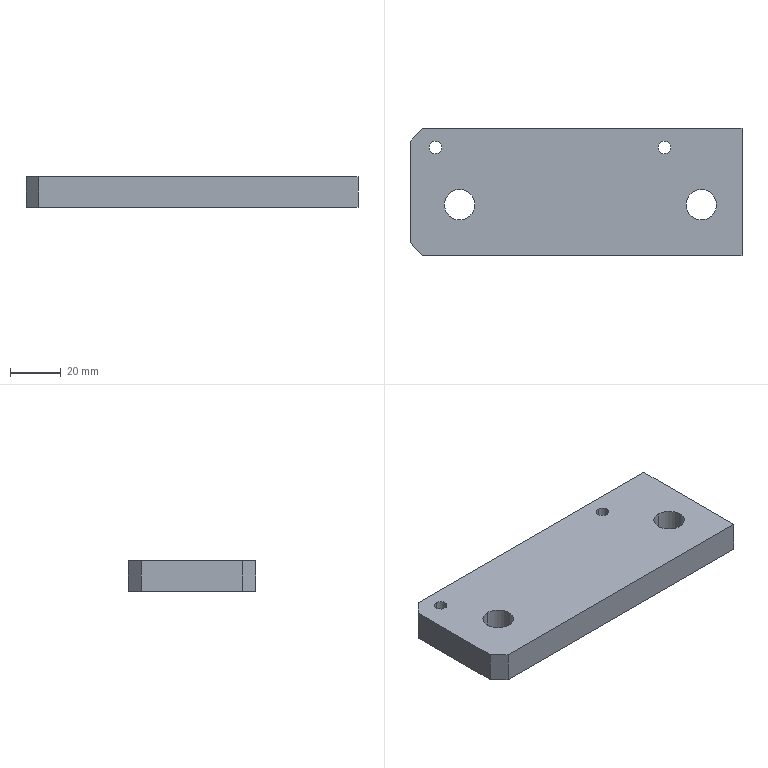Part | STEP file | [12] | 1 solid | 16 faces | box 130.5 x 50 x 12 mm | volume 74814 mm3 | cylinder 8 | plane 8 | commonest cylinder face diameters 5 x4 12 x4
STEP:
#1=CARTESIAN_POINT('',(100.,45.,12.));
#2=VERTEX_POINT('',#1);
#3=CARTESIAN_POINT('',(100.,40.,12.));
#4=VERTEX_POINT('',#3);
#5=CARTESIAN_POINT('',(100.,42.5,12.));
#6=DIRECTION('',(0.,0.,-1.));
#7=DIRECTION('',(0.,-1.,0.));
#8=AXIS2_PLACEMENT_3D('',#5,#6,#7);
#9=CIRCLE('',#8,2.5);
#10=EDGE_CURVE('',#2,#4,#9,.T.);
#11=ORIENTED_EDGE('',*,*,#10,.F.);
#12=CARTESIAN_POINT('',(100.,45.,0.));
#13=VERTEX_POINT('',#12);
#14=CARTESIAN_POINT('',(100.,45.,12.));
#15=DIRECTION('',(0.,0.,-1.));
#16=VECTOR('',#15,1000.);
#17=LINE('',#14,#16);
#18=EDGE_CURVE('',#2,#13,#17,.T.);
#19=ORIENTED_EDGE('',*,*,#18,.T.);
#20=CARTESIAN_POINT('',(100.,40.,0.));
#21=VERTEX_POINT('',#20);
#22=CARTESIAN_POINT('',(100.,42.5,0.));
#23=DIRECTION('',(0.,0.,1.));
#24=DIRECTION('',(0.,1.,0.));
#25=AXIS2_PLACEMENT_3D('',#22,#23,#24);
#26=CIRCLE('',#25,2.5);
#27=EDGE_CURVE('',#21,#13,#26,.T.);
#28=ORIENTED_EDGE('',*,*,#27,.F.);
#29=CARTESIAN_POINT('',(100.,40.,12.));
#30=DIRECTION('',(0.,0.,-1.));
#31=VECTOR('',#30,1000.);
#32=LINE('',#29,#31);
#33=EDGE_CURVE('',#4,#21,#32,.T.);
#34=ORIENTED_EDGE('',*,*,#33,.F.);
#35=EDGE_LOOP('',(#11,#19,#28,#34));
#36=FACE_OUTER_BOUND('',#35,.T.);
#37=CARTESIAN_POINT('',(100.,42.5,12.));
#38=DIRECTION('',(0.,0.,-1.));
#39=DIRECTION('',(0.,-1.,0.));
#40=AXIS2_PLACEMENT_3D('',#37,#38,#39);
#41=CYLINDRICAL_SURFACE('',#40,2.5);
#42=ADVANCED_FACE('',(#36),#41,.F.);
#43=CARTESIAN_POINT('',(10.,45.,12.));
#44=VERTEX_POINT('',#43);
#45=CARTESIAN_POINT('',(10.,40.,12.));
#46=VERTEX_POINT('',#45);
#47=CARTESIAN_POINT('',(10.,42.5,12.));
#48=DIRECTION('',(0.,0.,-1.));
#49=DIRECTION('',(0.,-1.,0.));
#50=AXIS2_PLACEMENT_3D('',#47,#48,#49);
#51=CIRCLE('',#50,2.5);
#52=EDGE_CURVE('',#44,#46,#51,.T.);
#53=ORIENTED_EDGE('',*,*,#52,.F.);
#54=CARTESIAN_POINT('',(10.,45.,0.));
#55=VERTEX_POINT('',#54);
#56=CARTESIAN_POINT('',(10.,45.,12.));
#57=DIRECTION('',(0.,0.,-1.));
#58=VECTOR('',#57,1000.);
#59=LINE('',#56,#58);
#60=EDGE_CURVE('',#44,#55,#59,.T.);
#61=ORIENTED_EDGE('',*,*,#60,.T.);
#62=CARTESIAN_POINT('',(10.,40.,0.));
#63=VERTEX_POINT('',#62);
#64=CARTESIAN_POINT('',(10.,42.5,0.));
#65=DIRECTION('',(0.,0.,1.));
#66=DIRECTION('',(0.,1.,0.));
#67=AXIS2_PLACEMENT_3D('',#64,#65,#66);
#68=CIRCLE('',#67,2.5);
#69=EDGE_CURVE('',#63,#55,#68,.T.);
#70=ORIENTED_EDGE('',*,*,#69,.F.);
#71=CARTESIAN_POINT('',(10.,40.,12.));
#72=DIRECTION('',(0.,0.,-1.));
#73=VECTOR('',#72,1000.);
#74=LINE('',#71,#73);
#75=EDGE_CURVE('',#46,#63,#74,.T.);
#76=ORIENTED_EDGE('',*,*,#75,.F.);
#77=EDGE_LOOP('',(#53,#61,#70,#76));
#78=FACE_OUTER_BOUND('',#77,.T.);
#79=CARTESIAN_POINT('',(10.,42.5,12.));
#80=DIRECTION('',(0.,0.,-1.));
#81=DIRECTION('',(0.,-1.,0.));
#82=AXIS2_PLACEMENT_3D('',#79,#80,#81);
#83=CYLINDRICAL_SURFACE('',#82,2.5);
#84=ADVANCED_FACE('',(#78),#83,.F.);
#85=CARTESIAN_POINT('',(114.5,26.,12.));
#86=VERTEX_POINT('',#85);
#87=CARTESIAN_POINT('',(114.5,14.,12.));
#88=VERTEX_POINT('',#87);
#89=CARTESIAN_POINT('',(114.5,20.,12.));
#90=DIRECTION('',(0.,0.,-1.));
#91=DIRECTION('',(0.,-1.,0.));
#92=AXIS2_PLACEMENT_3D('',#89,#90,#91);
#93=CIRCLE('',#92,6.);
#94=EDGE_CURVE('',#86,#88,#93,.T.);
#95=ORIENTED_EDGE('',*,*,#94,.F.);
#96=CARTESIAN_POINT('',(114.5,26.,0.));
#97=VERTEX_POINT('',#96);
#98=CARTESIAN_POINT('',(114.5,26.,12.));
#99=DIRECTION('',(0.,0.,-1.));
#100=VECTOR('',#99,1000.);
#101=LINE('',#98,#100);
#102=EDGE_CURVE('',#86,#97,#101,.T.);
#103=ORIENTED_EDGE('',*,*,#102,.T.);
#104=CARTESIAN_POINT('',(114.5,14.,0.));
#105=VERTEX_POINT('',#104);
#106=CARTESIAN_POINT('',(114.5,20.,0.));
#107=DIRECTION('',(0.,0.,1.));
#108=DIRECTION('',(0.,1.,0.));
#109=AXIS2_PLACEMENT_3D('',#106,#107,#108);
#110=CIRCLE('',#109,6.);
#111=EDGE_CURVE('',#105,#97,#110,.T.);
#112=ORIENTED_EDGE('',*,*,#111,.F.);
#113=CARTESIAN_POINT('',(114.5,14.,12.));
#114=DIRECTION('',(0.,0.,-1.));
#115=VECTOR('',#114,1000.);
#116=LINE('',#113,#115);
#117=EDGE_CURVE('',#88,#105,#116,.T.);
#118=ORIENTED_EDGE('',*,*,#117,.F.);
#119=EDGE_LOOP('',(#95,#103,#112,#118));
#120=FACE_OUTER_BOUND('',#119,.T.);
#121=CARTESIAN_POINT('',(114.5,20.,12.));
#122=DIRECTION('',(0.,0.,-1.));
#123=DIRECTION('',(0.,-1.,0.));
#124=AXIS2_PLACEMENT_3D('',#121,#122,#123);
#125=CYLINDRICAL_SURFACE('',#124,6.);
#126=ADVANCED_FACE('',(#120),#125,.F.);
#127=CARTESIAN_POINT('',(19.5,26.,12.));
#128=VERTEX_POINT('',#127);
#129=CARTESIAN_POINT('',(19.5,14.,12.));
#130=VERTEX_POINT('',#129);
#131=CARTESIAN_POINT('',(19.5,20.,12.));
#132=DIRECTION('',(0.,0.,-1.));
#133=DIRECTION('',(0.,-1.,0.));
#134=AXIS2_PLACEMENT_3D('',#131,#132,#133);
#135=CIRCLE('',#134,6.);
#136=EDGE_CURVE('',#128,#130,#135,.T.);
#137=ORIENTED_EDGE('',*,*,#136,.F.);
#138=CARTESIAN_POINT('',(19.5,26.,0.));
#139=VERTEX_POINT('',#138);
#140=CARTESIAN_POINT('',(19.5,26.,12.));
#141=DIRECTION('',(0.,0.,-1.));
#142=VECTOR('',#141,1000.);
#143=LINE('',#140,#142);
#144=EDGE_CURVE('',#128,#139,#143,.T.);
#145=ORIENTED_EDGE('',*,*,#144,.T.);
#146=CARTESIAN_POINT('',(19.5,14.,0.));
#147=VERTEX_POINT('',#146);
#148=CARTESIAN_POINT('',(19.5,20.,0.));
#149=DIRECTION('',(0.,0.,1.));
#150=DIRECTION('',(0.,1.,0.));
#151=AXIS2_PLACEMENT_3D('',#148,#149,#150);
#152=CIRCLE('',#151,6.);
#153=EDGE_CURVE('',#147,#139,#152,.T.);
#154=ORIENTED_EDGE('',*,*,#153,.F.);
#155=CARTESIAN_POINT('',(19.5,14.,12.));
#156=DIRECTION('',(0.,0.,-1.));
#157=VECTOR('',#156,1000.);
#158=LINE('',#155,#157);
#159=EDGE_CURVE('',#130,#147,#158,.T.);
#160=ORIENTED_EDGE('',*,*,#159,.F.);
#161=EDGE_LOOP('',(#137,#145,#154,#160));
#162=FACE_OUTER_BOUND('',#161,.T.);
#163=CARTESIAN_POINT('',(19.5,20.,12.));
#164=DIRECTION('',(0.,0.,-1.));
#165=DIRECTION('',(0.,-1.,0.));
#166=AXIS2_PLACEMENT_3D('',#163,#164,#165);
#167=CYLINDRICAL_SURFACE('',#166,6.);
#168=ADVANCED_FACE('',(#162),#167,.F.);
#169=CARTESIAN_POINT('',(100.,42.5,12.));
#170=DIRECTION('',(0.,0.,-1.));
#171=DIRECTION('',(0.,-1.,0.));
#172=AXIS2_PLACEMENT_3D('',#169,#170,#171);
#173=CIRCLE('',#172,2.5);
#174=EDGE_CURVE('',#4,#2,#173,.T.);
#175=ORIENTED_EDGE('',*,*,#174,.T.);
#176=ORIENTED_EDGE('',*,*,#10,.T.);
#177=EDGE_LOOP('',(#175,#176));
#178=FACE_BOUND('',#177,.T.);
#179=CARTESIAN_POINT('',(10.,42.5,12.));
#180=DIRECTION('',(0.,0.,-1.));
#181=DIRECTION('',(0.,-1.,0.));
#182=AXIS2_PLACEMENT_3D('',#179,#180,#181);
#183=CIRCLE('',#182,2.5);
#184=EDGE_CURVE('',#46,#44,#183,.T.);
#185=ORIENTED_EDGE('',*,*,#184,.T.);
#186=ORIENTED_EDGE('',*,*,#52,.T.);
#187=EDGE_LOOP('',(#185,#186));
#188=FACE_BOUND('',#187,.T.);
#189=CARTESIAN_POINT('',(114.5,20.,12.));
#190=DIRECTION('',(0.,0.,-1.));
#191=DIRECTION('',(0.,-1.,0.));
#192=AXIS2_PLACEMENT_3D('',#189,#190,#191);
#193=CIRCLE('',#192,6.);
#194=EDGE_CURVE('',#88,#86,#193,.T.);
#195=ORIENTED_EDGE('',*,*,#194,.T.);
#196=ORIENTED_EDGE('',*,*,#94,.T.);
#197=EDGE_LOOP('',(#195,#196));
#198=FACE_BOUND('',#197,.T.);
#199=CARTESIAN_POINT('',(19.5,20.,12.));
#200=DIRECTION('',(0.,0.,-1.));
#201=DIRECTION('',(0.,-1.,0.));
#202=AXIS2_PLACEMENT_3D('',#199,#200,#201);
#203=CIRCLE('',#202,6.);
#204=EDGE_CURVE('',#130,#128,#203,.T.);
#205=ORIENTED_EDGE('',*,*,#204,.T.);
#206=ORIENTED_EDGE('',*,*,#136,.T.);
#207=EDGE_LOOP('',(#205,#206));
#208=FACE_BOUND('',#207,.T.);
#209=CARTESIAN_POINT('',(5.,50.,12.));
#210=VERTEX_POINT('',#209);
#211=CARTESIAN_POINT('',(130.5,50.,12.));
#212=VERTEX_POINT('',#211);
#213=CARTESIAN_POINT('',(65.25,50.,12.));
#214=DIRECTION('',(1.,0.,0.));
#215=VECTOR('',#214,1000.);
#216=LINE('',#213,#215);
#217=EDGE_CURVE('',#210,#212,#216,.T.);
#218=ORIENTED_EDGE('',*,*,#217,.F.);
#219=CARTESIAN_POINT('',(0.,45.,12.));
#220=VERTEX_POINT('',#219);
#221=CARTESIAN_POINT('',(22.625,67.625,12.));
#222=DIRECTION('',(-0.7071,-0.7071,0.));
#223=VECTOR('',#222,1000.);
#224=LINE('',#221,#223);
#225=EDGE_CURVE('',#210,#220,#224,.T.);
#226=ORIENTED_EDGE('',*,*,#225,.T.);
#227=CARTESIAN_POINT('',(0.,5.,12.));
#228=VERTEX_POINT('',#227);
#229=CARTESIAN_POINT('',(0.,25.,12.));
#230=DIRECTION('',(0.,1.,0.));
#231=VECTOR('',#230,1000.);
#232=LINE('',#229,#231);
#233=EDGE_CURVE('',#228,#220,#232,.T.);
#234=ORIENTED_EDGE('',*,*,#233,.F.);
#235=CARTESIAN_POINT('',(5.,0.,12.));
#236=VERTEX_POINT('',#235);
#237=CARTESIAN_POINT('',(22.625,-17.625,12.));
#238=DIRECTION('',(0.7071,-0.7071,0.));
#239=VECTOR('',#238,1000.);
#240=LINE('',#237,#239);
#241=EDGE_CURVE('',#228,#236,#240,.T.);
#242=ORIENTED_EDGE('',*,*,#241,.T.);
#243=CARTESIAN_POINT('',(130.5,0.,12.));
#244=VERTEX_POINT('',#243);
#245=CARTESIAN_POINT('',(65.25,0.,12.));
#246=DIRECTION('',(-1.,0.,0.));
#247=VECTOR('',#246,1000.);
#248=LINE('',#245,#247);
#249=EDGE_CURVE('',#244,#236,#248,.T.);
#250=ORIENTED_EDGE('',*,*,#249,.F.);
#251=CARTESIAN_POINT('',(130.5,25.,12.));
#252=DIRECTION('',(0.,-1.,0.));
#253=VECTOR('',#252,1000.);
#254=LINE('',#251,#253);
#255=EDGE_CURVE('',#212,#244,#254,.T.);
#256=ORIENTED_EDGE('',*,*,#255,.F.);
#257=EDGE_LOOP('',(#218,#226,#234,#242,#250,#256));
#258=FACE_OUTER_BOUND('',#257,.T.);
#259=CARTESIAN_POINT('',(65.25,25.,12.));
#260=DIRECTION('',(0.,0.,1.));
#261=DIRECTION('',(-1.,0.,0.));
#262=AXIS2_PLACEMENT_3D('',#259,#260,#261);
#263=PLANE('',#262);
#264=ADVANCED_FACE('',(#178,#188,#198,#208,#258),#263,.T.);
#265=CARTESIAN_POINT('',(130.5,50.,0.));
#266=VERTEX_POINT('',#265);
#267=CARTESIAN_POINT('',(5.,50.,0.));
#268=VERTEX_POINT('',#267);
#269=CARTESIAN_POINT('',(65.25,50.,0.));
#270=DIRECTION('',(-1.,0.,0.));
#271=VECTOR('',#270,1000.);
#272=LINE('',#269,#271);
#273=EDGE_CURVE('',#266,#268,#272,.T.);
#274=ORIENTED_EDGE('',*,*,#273,.T.);
#275=CARTESIAN_POINT('',(5.,50.,0.));
#276=DIRECTION('',(0.,0.,1.));
#277=VECTOR('',#276,1000.);
#278=LINE('',#275,#277);
#279=EDGE_CURVE('',#268,#210,#278,.T.);
#280=ORIENTED_EDGE('',*,*,#279,.T.);
#281=ORIENTED_EDGE('',*,*,#217,.T.);
#282=CARTESIAN_POINT('',(130.5,50.,0.));
#283=DIRECTION('',(0.,0.,1.));
#284=VECTOR('',#283,1000.);
#285=LINE('',#282,#284);
#286=EDGE_CURVE('',#266,#212,#285,.T.);
#287=ORIENTED_EDGE('',*,*,#286,.F.);
#288=EDGE_LOOP('',(#274,#280,#281,#287));
#289=FACE_OUTER_BOUND('',#288,.T.);
#290=CARTESIAN_POINT('',(65.25,50.,0.));
#291=DIRECTION('',(0.,1.,0.));
#292=DIRECTION('',(0.,0.,-1.));
#293=AXIS2_PLACEMENT_3D('',#290,#291,#292);
#294=PLANE('',#293);
#295=ADVANCED_FACE('',(#289),#294,.T.);
#296=ORIENTED_EDGE('',*,*,#286,.T.);
#297=ORIENTED_EDGE('',*,*,#255,.T.);
#298=CARTESIAN_POINT('',(130.5,0.,0.));
#299=VERTEX_POINT('',#298);
#300=CARTESIAN_POINT('',(130.5,0.,0.));
#301=DIRECTION('',(0.,0.,1.));
#302=VECTOR('',#301,1000.);
#303=LINE('',#300,#302);
#304=EDGE_CURVE('',#299,#244,#303,.T.);
#305=ORIENTED_EDGE('',*,*,#304,.F.);
#306=CARTESIAN_POINT('',(130.5,25.,0.));
#307=DIRECTION('',(0.,1.,0.));
#308=VECTOR('',#307,1000.);
#309=LINE('',#306,#308);
#310=EDGE_CURVE('',#299,#266,#309,.T.);
#311=ORIENTED_EDGE('',*,*,#310,.T.);
#312=EDGE_LOOP('',(#296,#297,#305,#311));
#313=FACE_OUTER_BOUND('',#312,.T.);
#314=CARTESIAN_POINT('',(130.5,25.,0.));
#315=DIRECTION('',(1.,0.,0.));
#316=DIRECTION('',(0.,0.,1.));
#317=AXIS2_PLACEMENT_3D('',#314,#315,#316);
#318=PLANE('',#317);
#319=ADVANCED_FACE('',(#313),#318,.T.);
#320=ORIENTED_EDGE('',*,*,#249,.T.);
#321=CARTESIAN_POINT('',(5.,0.,0.));
#322=VERTEX_POINT('',#321);
#323=CARTESIAN_POINT('',(5.,0.,0.));
#324=DIRECTION('',(0.,0.,-1.));
#325=VECTOR('',#324,1000.);
#326=LINE('',#323,#325);
#327=EDGE_CURVE('',#236,#322,#326,.T.);
#328=ORIENTED_EDGE('',*,*,#327,.T.);
#329=CARTESIAN_POINT('',(65.25,0.,0.));
#330=DIRECTION('',(1.,0.,0.));
#331=VECTOR('',#330,1000.);
#332=LINE('',#329,#331);
#333=EDGE_CURVE('',#322,#299,#332,.T.);
#334=ORIENTED_EDGE('',*,*,#333,.T.);
#335=ORIENTED_EDGE('',*,*,#304,.T.);
#336=EDGE_LOOP('',(#320,#328,#334,#335));
#337=FACE_OUTER_BOUND('',#336,.T.);
#338=CARTESIAN_POINT('',(65.25,0.,0.));
#339=DIRECTION('',(0.,-1.,0.));
#340=DIRECTION('',(0.,0.,1.));
#341=AXIS2_PLACEMENT_3D('',#338,#339,#340);
#342=PLANE('',#341);
#343=ADVANCED_FACE('',(#337),#342,.T.);
#344=ORIENTED_EDGE('',*,*,#27,.T.);
#345=CARTESIAN_POINT('',(100.,42.5,0.));
#346=DIRECTION('',(0.,0.,1.));
#347=DIRECTION('',(0.,1.,0.));
#348=AXIS2_PLACEMENT_3D('',#345,#346,#347);
#349=CIRCLE('',#348,2.5);
#350=EDGE_CURVE('',#13,#21,#349,.T.);
#351=ORIENTED_EDGE('',*,*,#350,.T.);
#352=EDGE_LOOP('',(#344,#351));
#353=FACE_BOUND('',#352,.T.);
#354=ORIENTED_EDGE('',*,*,#69,.T.);
#355=CARTESIAN_POINT('',(10.,42.5,0.));
#356=DIRECTION('',(0.,0.,1.));
#357=DIRECTION('',(0.,1.,0.));
#358=AXIS2_PLACEMENT_3D('',#355,#356,#357);
#359=CIRCLE('',#358,2.5);
#360=EDGE_CURVE('',#55,#63,#359,.T.);
#361=ORIENTED_EDGE('',*,*,#360,.T.);
#362=EDGE_LOOP('',(#354,#361));
#363=FACE_BOUND('',#362,.T.);
#364=ORIENTED_EDGE('',*,*,#111,.T.);
#365=CARTESIAN_POINT('',(114.5,20.,0.));
#366=DIRECTION('',(0.,0.,1.));
#367=DIRECTION('',(0.,1.,0.));
#368=AXIS2_PLACEMENT_3D('',#365,#366,#367);
#369=CIRCLE('',#368,6.);
#370=EDGE_CURVE('',#97,#105,#369,.T.);
#371=ORIENTED_EDGE('',*,*,#370,.T.);
#372=EDGE_LOOP('',(#364,#371));
#373=FACE_BOUND('',#372,.T.);
#374=ORIENTED_EDGE('',*,*,#153,.T.);
#375=CARTESIAN_POINT('',(19.5,20.,0.));
#376=DIRECTION('',(0.,0.,1.));
#377=DIRECTION('',(0.,1.,0.));
#378=AXIS2_PLACEMENT_3D('',#375,#376,#377);
#379=CIRCLE('',#378,6.);
#380=EDGE_CURVE('',#139,#147,#379,.T.);
#381=ORIENTED_EDGE('',*,*,#380,.T.);
#382=EDGE_LOOP('',(#374,#381));
#383=FACE_BOUND('',#382,.T.);
#384=CARTESIAN_POINT('',(0.,45.,0.));
#385=VERTEX_POINT('',#384);
#386=CARTESIAN_POINT('',(0.,5.,0.));
#387=VERTEX_POINT('',#386);
#388=CARTESIAN_POINT('',(0.,25.,0.));
#389=DIRECTION('',(0.,-1.,0.));
#390=VECTOR('',#389,1000.);
#391=LINE('',#388,#390);
#392=EDGE_CURVE('',#385,#387,#391,.T.);
#393=ORIENTED_EDGE('',*,*,#392,.F.);
#394=CARTESIAN_POINT('',(22.625,67.625,0.));
#395=DIRECTION('',(0.7071,0.7071,0.));
#396=VECTOR('',#395,1000.);
#397=LINE('',#394,#396);
#398=EDGE_CURVE('',#385,#268,#397,.T.);
#399=ORIENTED_EDGE('',*,*,#398,.T.);
#400=ORIENTED_EDGE('',*,*,#273,.F.);
#401=ORIENTED_EDGE('',*,*,#310,.F.);
#402=ORIENTED_EDGE('',*,*,#333,.F.);
#403=CARTESIAN_POINT('',(22.625,-17.625,0.));
#404=DIRECTION('',(-0.7071,0.7071,0.));
#405=VECTOR('',#404,1000.);
#406=LINE('',#403,#405);
#407=EDGE_CURVE('',#322,#387,#406,.T.);
#408=ORIENTED_EDGE('',*,*,#407,.T.);
#409=EDGE_LOOP('',(#393,#399,#400,#401,#402,#408));
#410=FACE_OUTER_BOUND('',#409,.T.);
#411=CARTESIAN_POINT('',(65.25,25.,0.));
#412=DIRECTION('',(0.,0.,-1.));
#413=DIRECTION('',(1.,0.,0.));
#414=AXIS2_PLACEMENT_3D('',#411,#412,#413);
#415=PLANE('',#414);
#416=ADVANCED_FACE('',(#353,#363,#373,#383,#410),#415,.T.);
#417=ORIENTED_EDGE('',*,*,#233,.T.);
#418=CARTESIAN_POINT('',(0.,45.,0.));
#419=DIRECTION('',(0.,0.,-1.));
#420=VECTOR('',#419,1000.);
#421=LINE('',#418,#420);
#422=EDGE_CURVE('',#220,#385,#421,.T.);
#423=ORIENTED_EDGE('',*,*,#422,.T.);
#424=ORIENTED_EDGE('',*,*,#392,.T.);
#425=CARTESIAN_POINT('',(0.,5.,0.));
#426=DIRECTION('',(0.,0.,1.));
#427=VECTOR('',#426,1000.);
#428=LINE('',#425,#427);
#429=EDGE_CURVE('',#387,#228,#428,.T.);
#430=ORIENTED_EDGE('',*,*,#429,.T.);
#431=EDGE_LOOP('',(#417,#423,#424,#430));
#432=FACE_OUTER_BOUND('',#431,.T.);
#433=CARTESIAN_POINT('',(0.,25.,0.));
#434=DIRECTION('',(-1.,0.,0.));
#435=DIRECTION('',(0.,0.,-1.));
#436=AXIS2_PLACEMENT_3D('',#433,#434,#435);
#437=PLANE('',#436);
#438=ADVANCED_FACE('',(#432),#437,.T.);
#439=ORIENTED_EDGE('',*,*,#144,.F.);
#440=ORIENTED_EDGE('',*,*,#204,.F.);
#441=ORIENTED_EDGE('',*,*,#159,.T.);
#442=ORIENTED_EDGE('',*,*,#380,.F.);
#443=EDGE_LOOP('',(#439,#440,#441,#442));
#444=FACE_OUTER_BOUND('',#443,.T.);
#445=CARTESIAN_POINT('',(19.5,20.,12.));
#446=DIRECTION('',(0.,0.,-1.));
#447=DIRECTION('',(0.,-1.,0.));
#448=AXIS2_PLACEMENT_3D('',#445,#446,#447);
#449=CYLINDRICAL_SURFACE('',#448,6.);
#450=ADVANCED_FACE('',(#444),#449,.F.);
#451=ORIENTED_EDGE('',*,*,#102,.F.);
#452=ORIENTED_EDGE('',*,*,#194,.F.);
#453=ORIENTED_EDGE('',*,*,#117,.T.);
#454=ORIENTED_EDGE('',*,*,#370,.F.);
#455=EDGE_LOOP('',(#451,#452,#453,#454));
#456=FACE_OUTER_BOUND('',#455,.T.);
#457=CARTESIAN_POINT('',(114.5,20.,12.));
#458=DIRECTION('',(0.,0.,-1.));
#459=DIRECTION('',(0.,-1.,0.));
#460=AXIS2_PLACEMENT_3D('',#457,#458,#459);
#461=CYLINDRICAL_SURFACE('',#460,6.);
#462=ADVANCED_FACE('',(#456),#461,.F.);
#463=ORIENTED_EDGE('',*,*,#407,.F.);
#464=ORIENTED_EDGE('',*,*,#327,.F.);
#465=ORIENTED_EDGE('',*,*,#241,.F.);
#466=ORIENTED_EDGE('',*,*,#429,.F.);
#467=EDGE_LOOP('',(#463,#464,#465,#466));
#468=FACE_OUTER_BOUND('',#467,.T.);
#469=CARTESIAN_POINT('',(0.,5.,0.));
#470=DIRECTION('',(0.7071,0.7071,0.));
#471=DIRECTION('',(0.,0.,1.));
#472=AXIS2_PLACEMENT_3D('',#469,#470,#471);
#473=PLANE('',#472);
#474=ADVANCED_FACE('',(#468),#473,.F.);
#475=ORIENTED_EDGE('',*,*,#398,.F.);
#476=ORIENTED_EDGE('',*,*,#422,.F.);
#477=ORIENTED_EDGE('',*,*,#225,.F.);
#478=ORIENTED_EDGE('',*,*,#279,.F.);
#479=EDGE_LOOP('',(#475,#476,#477,#478));
#480=FACE_OUTER_BOUND('',#479,.T.);
#481=CARTESIAN_POINT('',(5.,50.,0.));
#482=DIRECTION('',(0.7071,-0.7071,0.));
#483=DIRECTION('',(0.,0.,1.));
#484=AXIS2_PLACEMENT_3D('',#481,#482,#483);
#485=PLANE('',#484);
#486=ADVANCED_FACE('',(#480),#485,.F.);
#487=ORIENTED_EDGE('',*,*,#60,.F.);
#488=ORIENTED_EDGE('',*,*,#184,.F.);
#489=ORIENTED_EDGE('',*,*,#75,.T.);
#490=ORIENTED_EDGE('',*,*,#360,.F.);
#491=EDGE_LOOP('',(#487,#488,#489,#490));
#492=FACE_OUTER_BOUND('',#491,.T.);
#493=CARTESIAN_POINT('',(10.,42.5,12.));
#494=DIRECTION('',(0.,0.,-1.));
#495=DIRECTION('',(0.,-1.,0.));
#496=AXIS2_PLACEMENT_3D('',#493,#494,#495);
#497=CYLINDRICAL_SURFACE('',#496,2.5);
#498=ADVANCED_FACE('',(#492),#497,.F.);
#499=ORIENTED_EDGE('',*,*,#18,.F.);
#500=ORIENTED_EDGE('',*,*,#174,.F.);
#501=ORIENTED_EDGE('',*,*,#33,.T.);
#502=ORIENTED_EDGE('',*,*,#350,.F.);
#503=EDGE_LOOP('',(#499,#500,#501,#502));
#504=FACE_OUTER_BOUND('',#503,.T.);
#505=CARTESIAN_POINT('',(100.,42.5,12.));
#506=DIRECTION('',(0.,0.,-1.));
#507=DIRECTION('',(0.,-1.,0.));
#508=AXIS2_PLACEMENT_3D('',#505,#506,#507);
#509=CYLINDRICAL_SURFACE('',#508,2.5);
#510=ADVANCED_FACE('',(#504),#509,.F.);
#511=CLOSED_SHELL('',(#42,#84,#126,#168,#264,#295,#319,#343,#416,#438,#450,#462,#474,#486,#498,#510));
#512=MANIFOLD_SOLID_BREP('',#511);
#513=CARTESIAN_POINT('',(0.,0.,0.));
#514=DIRECTION('',(0.,0.,1.));
#515=DIRECTION('',(1.,0.,0.));
#516=AXIS2_PLACEMENT_3D('',#513,#514,#515);
#517=(LENGTH_UNIT()NAMED_UNIT(*)SI_UNIT(.MILLI.,.METRE.));
#518=UNCERTAINTY_MEASURE_WITH_UNIT(LENGTH_MEASURE(0.00001),#517,'','');
#519=(NAMED_UNIT(*)PLANE_ANGLE_UNIT()SI_UNIT($,.RADIAN.));
#520=(NAMED_UNIT(*)SI_UNIT($,.STERADIAN.)SOLID_ANGLE_UNIT());
#521=(GEOMETRIC_REPRESENTATION_CONTEXT(3)GLOBAL_UNCERTAINTY_ASSIGNED_CONTEXT((#518))GLOBAL_UNIT_ASSIGNED_CONTEXT((#517,#519,#520))REPRESENTATION_CONTEXT('',''));
#522=ADVANCED_BREP_SHAPE_REPRESENTATION('',(#512,#516),#521);